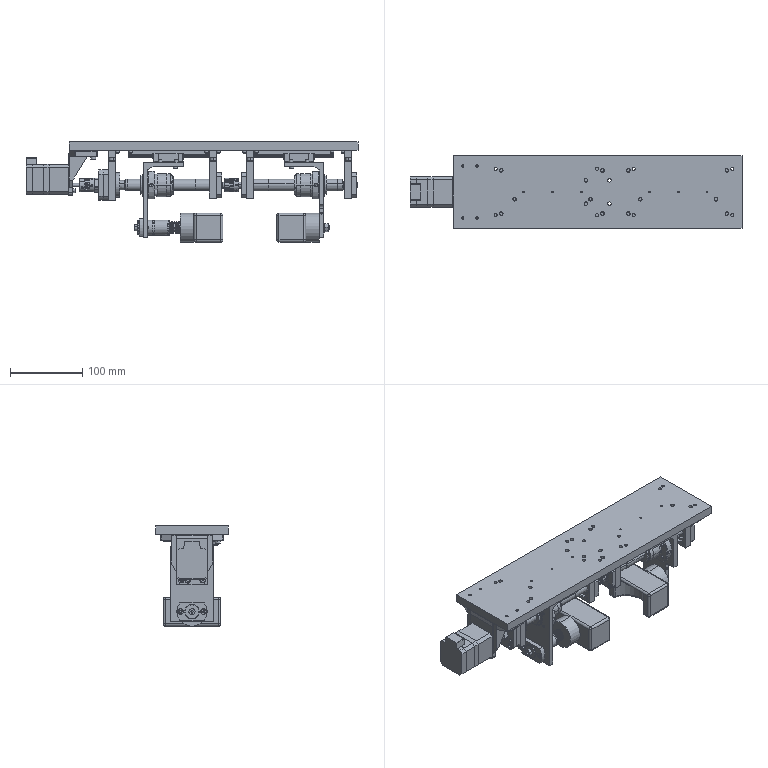Part | SolidWorks | features AEMSimFeature 1, CompositeCurve 1, MateUpdatePoint 1 | 87 solids | 3233 faces | volume 1293275 mm3 | plane 1633 | cylinder 1151 | cone 372 | sphere 56 | spline 11 | torus 10 | commonest cylinder face diameters 2.5 x94 5 x91 3.4 x62 0.4 x60 3.5 x52 6 x47